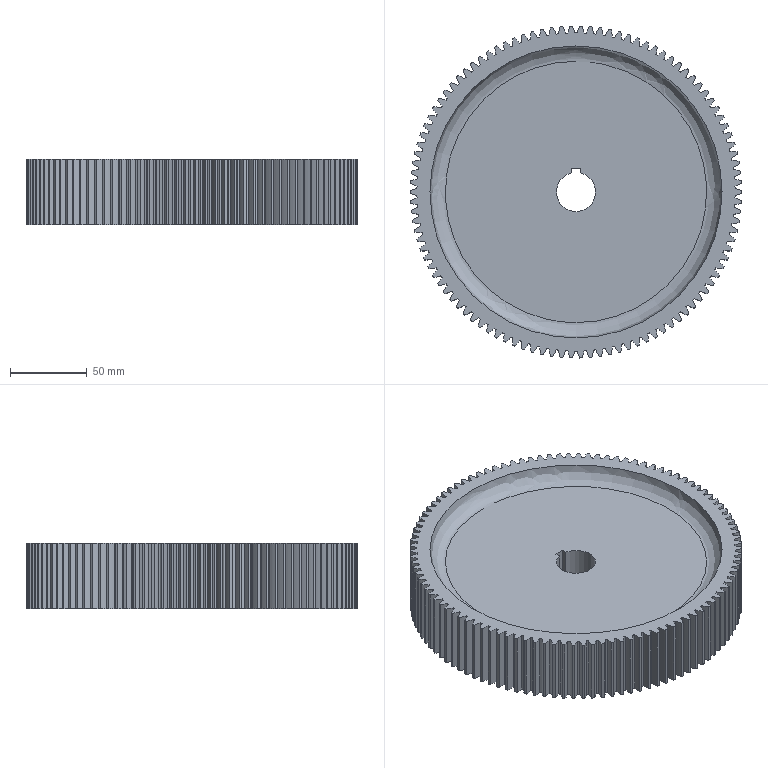Part | STEP file | GEAR2-2_id446_x_t | 1 solid | 434 faces | box 216 x 215.948 x 42.5 mm | volume 942512 mm3 | cylinder 425 | plane 7 | other 2 | commonest cylinder face diameters 70.905 x212 207 x106 216 x106 25.5 x1